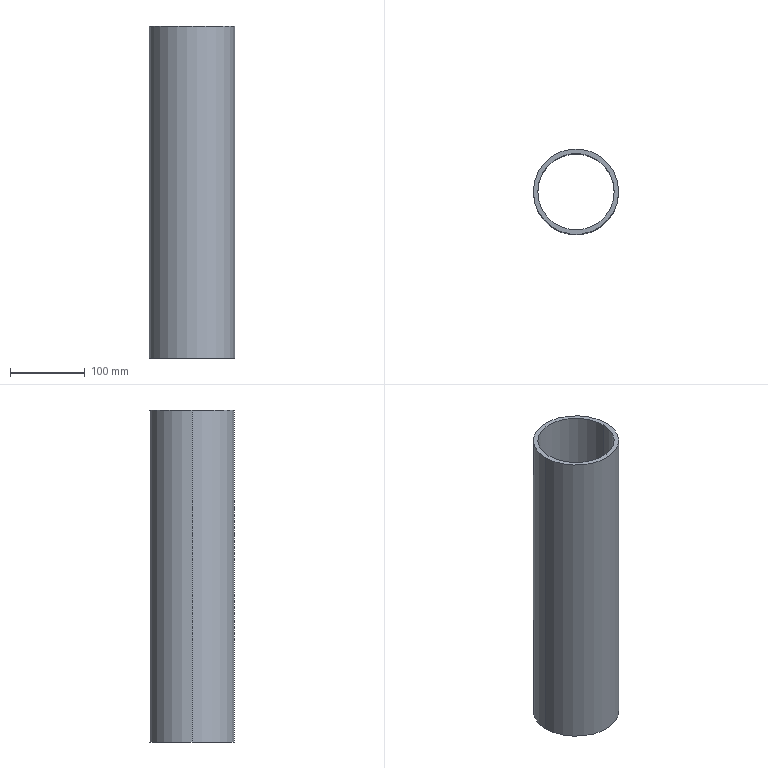Part | SolidWorks | features Extrusion 1 | 1 solid | 6 faces | box 114.3 x 114.3 x 444.5 mm | volume 910233 mm3 | cylinder 4 | plane 2 | commonest cylinder face diameters 102.26 x2 114.3 x2
STEP:
#1=CARTESIAN_POINT('',(-51.13,0.,222.25));
#2=VERTEX_POINT('',#1);
#3=CARTESIAN_POINT('',(51.13,0.,222.25));
#4=VERTEX_POINT('',#3);
#5=CARTESIAN_POINT('',(0.,0.,222.25));
#6=DIRECTION('',(0.,0.,1.));
#7=DIRECTION('',(1.,0.,0.));
#8=AXIS2_PLACEMENT_3D('',#5,#6,#7);
#9=CIRCLE('',#8,51.13);
#10=EDGE_CURVE('',#2,#4,#9,.T.);
#11=ORIENTED_EDGE('',*,*,#10,.T.);
#12=CARTESIAN_POINT('',(51.13,0.,-222.25));
#13=VERTEX_POINT('',#12);
#14=CARTESIAN_POINT('',(51.13,0.,222.25));
#15=DIRECTION('',(0.,0.,-1.));
#16=VECTOR('',#15,1000.);
#17=LINE('',#14,#16);
#18=EDGE_CURVE('',#4,#13,#17,.T.);
#19=ORIENTED_EDGE('',*,*,#18,.T.);
#20=CARTESIAN_POINT('',(-51.13,0.,-222.25));
#21=VERTEX_POINT('',#20);
#22=CARTESIAN_POINT('',(0.,0.,-222.25));
#23=DIRECTION('',(0.,0.,1.));
#24=DIRECTION('',(1.,0.,0.));
#25=AXIS2_PLACEMENT_3D('',#22,#23,#24);
#26=CIRCLE('',#25,51.13);
#27=EDGE_CURVE('',#21,#13,#26,.T.);
#28=ORIENTED_EDGE('',*,*,#27,.F.);
#29=CARTESIAN_POINT('',(-51.13,0.,222.25));
#30=DIRECTION('',(0.,0.,-1.));
#31=VECTOR('',#30,1000.);
#32=LINE('',#29,#31);
#33=EDGE_CURVE('',#2,#21,#32,.T.);
#34=ORIENTED_EDGE('',*,*,#33,.F.);
#35=EDGE_LOOP('',(#11,#19,#28,#34));
#36=FACE_OUTER_BOUND('',#35,.T.);
#37=CARTESIAN_POINT('',(0.,0.,222.25));
#38=DIRECTION('',(0.,0.,-1.));
#39=DIRECTION('',(-1.,0.,0.));
#40=AXIS2_PLACEMENT_3D('',#37,#38,#39);
#41=CYLINDRICAL_SURFACE('',#40,51.13);
#42=ADVANCED_FACE('',(#36),#41,.F.);
#43=CARTESIAN_POINT('',(57.15,0.,222.25));
#44=VERTEX_POINT('',#43);
#45=CARTESIAN_POINT('',(-57.15,0.,222.25));
#46=VERTEX_POINT('',#45);
#47=CARTESIAN_POINT('',(0.,0.,222.25));
#48=DIRECTION('',(0.,0.,1.));
#49=DIRECTION('',(1.,0.,0.));
#50=AXIS2_PLACEMENT_3D('',#47,#48,#49);
#51=CIRCLE('',#50,57.15);
#52=EDGE_CURVE('',#44,#46,#51,.T.);
#53=ORIENTED_EDGE('',*,*,#52,.F.);
#54=CARTESIAN_POINT('',(57.15,0.,-222.25));
#55=VERTEX_POINT('',#54);
#56=CARTESIAN_POINT('',(57.15,0.,222.25));
#57=DIRECTION('',(0.,0.,-1.));
#58=VECTOR('',#57,1000.);
#59=LINE('',#56,#58);
#60=EDGE_CURVE('',#44,#55,#59,.T.);
#61=ORIENTED_EDGE('',*,*,#60,.T.);
#62=CARTESIAN_POINT('',(-57.15,0.,-222.25));
#63=VERTEX_POINT('',#62);
#64=CARTESIAN_POINT('',(0.,0.,-222.25));
#65=DIRECTION('',(0.,0.,1.));
#66=DIRECTION('',(1.,0.,0.));
#67=AXIS2_PLACEMENT_3D('',#64,#65,#66);
#68=CIRCLE('',#67,57.15);
#69=EDGE_CURVE('',#55,#63,#68,.T.);
#70=ORIENTED_EDGE('',*,*,#69,.T.);
#71=CARTESIAN_POINT('',(-57.15,0.,222.25));
#72=DIRECTION('',(0.,0.,-1.));
#73=VECTOR('',#72,1000.);
#74=LINE('',#71,#73);
#75=EDGE_CURVE('',#46,#63,#74,.T.);
#76=ORIENTED_EDGE('',*,*,#75,.F.);
#77=EDGE_LOOP('',(#53,#61,#70,#76));
#78=FACE_OUTER_BOUND('',#77,.T.);
#79=CARTESIAN_POINT('',(0.,0.,222.25));
#80=DIRECTION('',(0.,0.,-1.));
#81=DIRECTION('',(-1.,0.,0.));
#82=AXIS2_PLACEMENT_3D('',#79,#80,#81);
#83=CYLINDRICAL_SURFACE('',#82,57.15);
#84=ADVANCED_FACE('',(#78),#83,.T.);
#85=CARTESIAN_POINT('',(0.,0.,222.25));
#86=DIRECTION('',(0.,0.,1.));
#87=DIRECTION('',(1.,0.,0.));
#88=AXIS2_PLACEMENT_3D('',#85,#86,#87);
#89=CIRCLE('',#88,57.15);
#90=EDGE_CURVE('',#46,#44,#89,.T.);
#91=ORIENTED_EDGE('',*,*,#90,.T.);
#92=ORIENTED_EDGE('',*,*,#52,.T.);
#93=EDGE_LOOP('',(#91,#92));
#94=FACE_OUTER_BOUND('',#93,.T.);
#95=ORIENTED_EDGE('',*,*,#10,.F.);
#96=CARTESIAN_POINT('',(0.,0.,222.25));
#97=DIRECTION('',(0.,0.,1.));
#98=DIRECTION('',(1.,0.,0.));
#99=AXIS2_PLACEMENT_3D('',#96,#97,#98);
#100=CIRCLE('',#99,51.13);
#101=EDGE_CURVE('',#4,#2,#100,.T.);
#102=ORIENTED_EDGE('',*,*,#101,.F.);
#103=EDGE_LOOP('',(#95,#102));
#104=FACE_BOUND('',#103,.T.);
#105=CARTESIAN_POINT('',(0.,0.,222.25));
#106=DIRECTION('',(0.,0.,1.));
#107=DIRECTION('',(1.,0.,0.));
#108=AXIS2_PLACEMENT_3D('',#105,#106,#107);
#109=PLANE('',#108);
#110=ADVANCED_FACE('',(#94,#104),#109,.T.);
#111=ORIENTED_EDGE('',*,*,#60,.F.);
#112=ORIENTED_EDGE('',*,*,#90,.F.);
#113=ORIENTED_EDGE('',*,*,#75,.T.);
#114=CARTESIAN_POINT('',(0.,0.,-222.25));
#115=DIRECTION('',(0.,0.,1.));
#116=DIRECTION('',(1.,0.,0.));
#117=AXIS2_PLACEMENT_3D('',#114,#115,#116);
#118=CIRCLE('',#117,57.15);
#119=EDGE_CURVE('',#63,#55,#118,.T.);
#120=ORIENTED_EDGE('',*,*,#119,.T.);
#121=EDGE_LOOP('',(#111,#112,#113,#120));
#122=FACE_OUTER_BOUND('',#121,.T.);
#123=CARTESIAN_POINT('',(0.,0.,222.25));
#124=DIRECTION('',(0.,0.,-1.));
#125=DIRECTION('',(-1.,0.,0.));
#126=AXIS2_PLACEMENT_3D('',#123,#124,#125);
#127=CYLINDRICAL_SURFACE('',#126,57.15);
#128=ADVANCED_FACE('',(#122),#127,.T.);
#129=ORIENTED_EDGE('',*,*,#18,.F.);
#130=ORIENTED_EDGE('',*,*,#101,.T.);
#131=ORIENTED_EDGE('',*,*,#33,.T.);
#132=CARTESIAN_POINT('',(0.,0.,-222.25));
#133=DIRECTION('',(0.,0.,1.));
#134=DIRECTION('',(1.,0.,0.));
#135=AXIS2_PLACEMENT_3D('',#132,#133,#134);
#136=CIRCLE('',#135,51.13);
#137=EDGE_CURVE('',#13,#21,#136,.T.);
#138=ORIENTED_EDGE('',*,*,#137,.F.);
#139=EDGE_LOOP('',(#129,#130,#131,#138));
#140=FACE_OUTER_BOUND('',#139,.T.);
#141=CARTESIAN_POINT('',(0.,0.,222.25));
#142=DIRECTION('',(0.,0.,-1.));
#143=DIRECTION('',(-1.,0.,0.));
#144=AXIS2_PLACEMENT_3D('',#141,#142,#143);
#145=CYLINDRICAL_SURFACE('',#144,51.13);
#146=ADVANCED_FACE('',(#140),#145,.F.);
#147=ORIENTED_EDGE('',*,*,#27,.T.);
#148=ORIENTED_EDGE('',*,*,#137,.T.);
#149=EDGE_LOOP('',(#147,#148));
#150=FACE_BOUND('',#149,.T.);
#151=ORIENTED_EDGE('',*,*,#119,.F.);
#152=ORIENTED_EDGE('',*,*,#69,.F.);
#153=EDGE_LOOP('',(#151,#152));
#154=FACE_OUTER_BOUND('',#153,.T.);
#155=CARTESIAN_POINT('',(0.,0.,-222.25));
#156=DIRECTION('',(0.,0.,1.));
#157=DIRECTION('',(1.,0.,0.));
#158=AXIS2_PLACEMENT_3D('',#155,#156,#157);
#159=PLANE('',#158);
#160=ADVANCED_FACE('',(#150,#154),#159,.F.);
#161=CLOSED_SHELL('',(#42,#84,#110,#128,#146,#160));
#162=MANIFOLD_SOLID_BREP('',#161);
#163=CARTESIAN_POINT('',(0.,0.,0.));
#164=DIRECTION('',(0.,0.,1.));
#165=DIRECTION('',(1.,0.,0.));
#166=AXIS2_PLACEMENT_3D('',#163,#164,#165);
#167=(LENGTH_UNIT()NAMED_UNIT(*)SI_UNIT(.MILLI.,.METRE.));
#168=UNCERTAINTY_MEASURE_WITH_UNIT(LENGTH_MEASURE(0.00001),#167,'','');
#169=(NAMED_UNIT(*)PLANE_ANGLE_UNIT()SI_UNIT($,.RADIAN.));
#170=(NAMED_UNIT(*)SI_UNIT($,.STERADIAN.)SOLID_ANGLE_UNIT());
#171=(GEOMETRIC_REPRESENTATION_CONTEXT(3)GLOBAL_UNCERTAINTY_ASSIGNED_CONTEXT((#168))GLOBAL_UNIT_ASSIGNED_CONTEXT((#167,#169,#170))REPRESENTATION_CONTEXT('',''));
#172=ADVANCED_BREP_SHAPE_REPRESENTATION('',(#162,#166),#171);